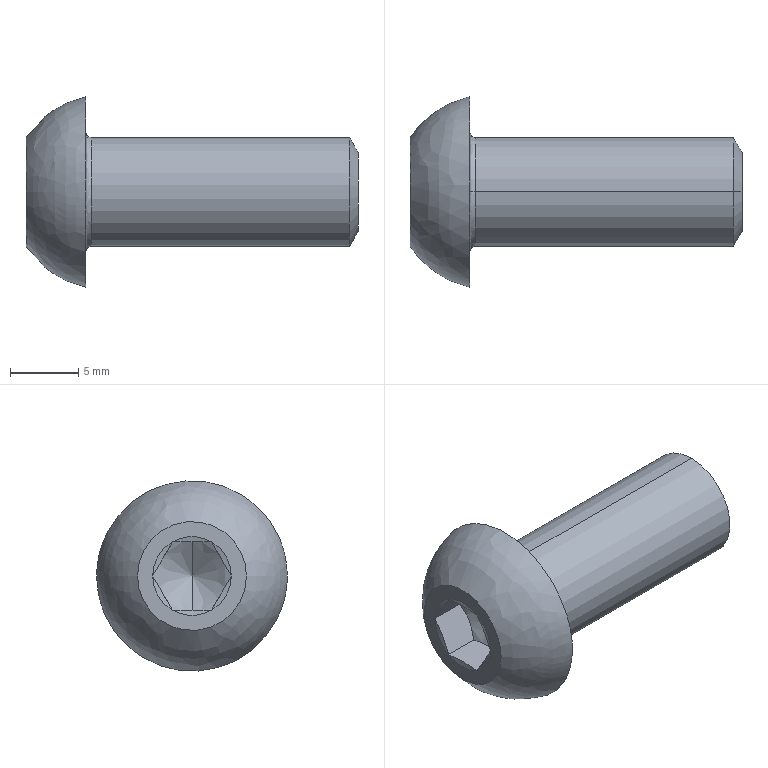Part | SolidWorks | features BaseBody 1 | 1 solid | 24 faces | box 24.4 x 14 x 14 mm | volume 1421 mm3 | cone 10 | plane 9 | spline 3 | cylinder 2 | commonest cylinder face diameters 8 x2
STEP:
#1=CARTESIAN_POINT('',(-19.6,0.,-4.));
#2=VERTEX_POINT('',#1);
#3=CARTESIAN_POINT('',(-19.6,0.,4.));
#4=VERTEX_POINT('',#3);
#5=CARTESIAN_POINT('',(-19.6,0.,0.));
#6=DIRECTION('',(1.,0.,0.));
#7=DIRECTION('',(0.,0.,1.));
#8=AXIS2_PLACEMENT_3D('',#5,#6,#7);
#9=CIRCLE('',#8,4.);
#10=EDGE_CURVE('',#2,#4,#9,.T.);
#11=ORIENTED_EDGE('',*,*,#10,.F.);
#12=CARTESIAN_POINT('',(-20.,0.,-4.4));
#13=VERTEX_POINT('',#12);
#14=CARTESIAN_POINT('',(-19.6,0.,-4.4));
#15=DIRECTION('',(0.,-1.,0.));
#16=DIRECTION('',(0.,0.,-1.));
#17=AXIS2_PLACEMENT_3D('',#14,#15,#16);
#18=CIRCLE('',#17,0.4);
#19=EDGE_CURVE('',#2,#13,#18,.T.);
#20=ORIENTED_EDGE('',*,*,#19,.T.);
#21=CARTESIAN_POINT('',(-20.,0.,4.4));
#22=VERTEX_POINT('',#21);
#23=CARTESIAN_POINT('',(-20.,0.,4.4));
#24=CARTESIAN_POINT('',(-20.,0.2798,4.4));
#25=CARTESIAN_POINT('',(-20.,0.6922,4.361));
#26=CARTESIAN_POINT('',(-20.,1.16,4.249));
#27=CARTESIAN_POINT('',(-20.,1.391,4.176));
#28=CARTESIAN_POINT('',(-20.,1.506,4.135));
#29=CARTESIAN_POINT('',(-20.,1.555,4.116));
#30=CARTESIAN_POINT('',(-20.,1.587,4.104));
#31=CARTESIAN_POINT('',(-20.,1.602,4.098));
#32=CARTESIAN_POINT('',(-20.,1.758,4.036));
#33=CARTESIAN_POINT('',(-20.,1.96,3.944));
#34=CARTESIAN_POINT('',(-20.,2.155,3.837));
#35=CARTESIAN_POINT('',(-20.,2.283,3.762));
#36=CARTESIAN_POINT('',(-20.,2.344,3.724));
#37=CARTESIAN_POINT('',(-20.,2.662,3.516));
#38=CARTESIAN_POINT('',(-20.,2.896,3.326));
#39=CARTESIAN_POINT('',(-20.,3.219,3.004));
#40=CARTESIAN_POINT('',(-20.,3.371,2.835));
#41=CARTESIAN_POINT('',(-20.,3.509,2.656));
#42=CARTESIAN_POINT('',(-20.,3.598,2.533));
#43=CARTESIAN_POINT('',(-20.,3.642,2.47));
#44=CARTESIAN_POINT('',(-20.,3.764,2.283));
#45=CARTESIAN_POINT('',(-20.,3.876,2.091));
#46=CARTESIAN_POINT('',(-20.,3.99,1.858));
#47=CARTESIAN_POINT('',(-20.,4.034,1.757));
#48=CARTESIAN_POINT('',(-20.,4.063,1.688));
#49=CARTESIAN_POINT('',(-20.,4.078,1.652));
#50=CARTESIAN_POINT('',(-20.,4.297,1.099));
#51=CARTESIAN_POINT('',(-20.,4.4,0.5599));
#52=CARTESIAN_POINT('',(-20.,4.4,-0.2799));
#53=CARTESIAN_POINT('',(-20.,4.361,-0.6923));
#54=CARTESIAN_POINT('',(-20.,4.249,-1.16));
#55=CARTESIAN_POINT('',(-20.,4.176,-1.391));
#56=CARTESIAN_POINT('',(-20.,4.135,-1.506));
#57=CARTESIAN_POINT('',(-20.,4.116,-1.555));
#58=CARTESIAN_POINT('',(-20.,4.104,-1.587));
#59=CARTESIAN_POINT('',(-20.,4.098,-1.602));
#60=CARTESIAN_POINT('',(-20.,4.036,-1.758));
#61=CARTESIAN_POINT('',(-20.,3.944,-1.96));
#62=CARTESIAN_POINT('',(-20.,3.837,-2.155));
#63=CARTESIAN_POINT('',(-20.,3.762,-2.283));
#64=CARTESIAN_POINT('',(-20.,3.724,-2.344));
#65=CARTESIAN_POINT('',(-20.,3.516,-2.662));
#66=CARTESIAN_POINT('',(-20.,3.326,-2.896));
#67=CARTESIAN_POINT('',(-20.,3.004,-3.219));
#68=CARTESIAN_POINT('',(-20.,2.835,-3.371));
#69=CARTESIAN_POINT('',(-20.,2.656,-3.509));
#70=CARTESIAN_POINT('',(-20.,2.533,-3.598));
#71=CARTESIAN_POINT('',(-20.,2.47,-3.642));
#72=CARTESIAN_POINT('',(-20.,2.283,-3.764));
#73=CARTESIAN_POINT('',(-20.,2.091,-3.876));
#74=CARTESIAN_POINT('',(-20.,1.858,-3.99));
#75=CARTESIAN_POINT('',(-20.,1.757,-4.034));
#76=CARTESIAN_POINT('',(-20.,1.688,-4.063));
#77=CARTESIAN_POINT('',(-20.,1.652,-4.078));
#78=CARTESIAN_POINT('',(-20.,1.099,-4.297));
#79=CARTESIAN_POINT('',(-20.,0.5593,-4.4));
#80=CARTESIAN_POINT('',(-20.,0.,-4.4));
#81=B_SPLINE_CURVE_WITH_KNOTS('',3,(#23,#24,#25,#26,#27,#28,#29,#30,#31,#32,#33,#34,#35,#36,#37,#38,#39,#40,#41,#42,#43,#44,#45,#46,#47,#48,#49,#50,#51,#52,#53,#54,#55,#56,#57,#58,#59,#60,#61,#62,#63,#64,#65,#66,#67,#68,#69,#70,#71,#72,#73,#74,#75,#76,#77,#78,#79,#80),.UNSPECIFIED.,.F.,.F.,(4,1,1,1,1,2,2,1,2,2,2,1,2,2,1,1,2,2,2,1,1,1,1,2,2,1,2,2,2,1,2,2,1,1,2,2,4),(0.,0.0625,0.09375,0.1094,0.1172,0.1211,0.125,0.1562,0.1719,0.1875,0.25,0.2812,0.2969,0.3125,0.3437,0.3594,0.3672,0.375,0.5,0.5625,0.5937,0.6094,0.6172,0.6211,0.625,0.6562,0.6719,0.6875,0.75,0.7812,0.7969,0.8125,0.8437,0.8594,0.8672,0.875,1.),.UNSPECIFIED.);
#82=EDGE_CURVE('',#22,#13,#81,.T.);
#83=ORIENTED_EDGE('',*,*,#82,.F.);
#84=CARTESIAN_POINT('',(-19.6,0.,4.4));
#85=DIRECTION('',(0.,1.,0.));
#86=DIRECTION('',(0.,0.,1.));
#87=AXIS2_PLACEMENT_3D('',#84,#85,#86);
#88=CIRCLE('',#87,0.4);
#89=EDGE_CURVE('',#4,#22,#88,.T.);
#90=ORIENTED_EDGE('',*,*,#89,.F.);
#91=EDGE_LOOP('',(#11,#20,#83,#90));
#92=FACE_OUTER_BOUND('',#91,.T.);
#93=CARTESIAN_POINT('',(-19.6,0.,4.));
#94=CARTESIAN_POINT('',(-19.6,8.,4.));
#95=CARTESIAN_POINT('',(-19.6,8.,-4.));
#96=CARTESIAN_POINT('',(-19.6,0.,-4.));
#97=CARTESIAN_POINT('',(-19.834,0.,4.));
#98=CARTESIAN_POINT('',(-19.834,8.,4.));
#99=CARTESIAN_POINT('',(-19.834,8.,-4.));
#100=CARTESIAN_POINT('',(-19.834,0.,-4.));
#101=CARTESIAN_POINT('',(-20.,0.,4.166));
#102=CARTESIAN_POINT('',(-20.,8.331,4.166));
#103=CARTESIAN_POINT('',(-20.,8.331,-4.166));
#104=CARTESIAN_POINT('',(-20.,0.,-4.166));
#105=CARTESIAN_POINT('',(-20.,0.,4.4));
#106=CARTESIAN_POINT('',(-20.,8.8,4.4));
#107=CARTESIAN_POINT('',(-20.,8.8,-4.4));
#108=CARTESIAN_POINT('',(-20.,0.,-4.4));
#109=(BOUNDED_SURFACE()B_SPLINE_SURFACE(3,3,((#93,#94,#95,#96),(#97,#98,#99,#100),(#101,#102,#103,#104),(#105,#106,#107,#108)),.UNSPECIFIED.,.F.,.F.,.F.)B_SPLINE_SURFACE_WITH_KNOTS((4,4),(4,4),(0.,1.),(0.,1.),.UNSPECIFIED.)GEOMETRIC_REPRESENTATION_ITEM()RATIONAL_B_SPLINE_SURFACE(((1.,0.3333,0.3333,1.),(0.8047,0.2682,0.2682,0.8047),(0.8047,0.2682,0.2682,0.8047),(1.,0.3333,0.3333,1.)))REPRESENTATION_ITEM('')SURFACE());
#110=ADVANCED_FACE('',(#92),#109,.F.);
#111=CARTESIAN_POINT('',(-0.625,0.,4.));
#112=VERTEX_POINT('',#111);
#113=CARTESIAN_POINT('',(-0.625,0.,-4.));
#114=VERTEX_POINT('',#113);
#115=CARTESIAN_POINT('',(-0.625,0.,0.));
#116=DIRECTION('',(-1.,0.,0.));
#117=DIRECTION('',(0.,0.,1.));
#118=AXIS2_PLACEMENT_3D('',#115,#116,#117);
#119=CIRCLE('',#118,4.);
#120=EDGE_CURVE('',#112,#114,#119,.T.);
#121=ORIENTED_EDGE('',*,*,#120,.T.);
#122=CARTESIAN_POINT('',(-24.4,0.,-4.));
#123=DIRECTION('',(-1.,0.,0.));
#124=VECTOR('',#123,1000.);
#125=LINE('',#122,#124);
#126=EDGE_CURVE('',#114,#2,#125,.T.);
#127=ORIENTED_EDGE('',*,*,#126,.T.);
#128=ORIENTED_EDGE('',*,*,#10,.T.);
#129=CARTESIAN_POINT('',(-24.4,0.,4.));
#130=DIRECTION('',(-1.,0.,0.));
#131=VECTOR('',#130,1000.);
#132=LINE('',#129,#131);
#133=EDGE_CURVE('',#112,#4,#132,.T.);
#134=ORIENTED_EDGE('',*,*,#133,.F.);
#135=EDGE_LOOP('',(#121,#127,#128,#134));
#136=FACE_OUTER_BOUND('',#135,.T.);
#137=CARTESIAN_POINT('',(-24.4,0.,0.));
#138=DIRECTION('',(-1.,0.,0.));
#139=DIRECTION('',(0.,0.,1.));
#140=AXIS2_PLACEMENT_3D('',#137,#138,#139);
#141=CYLINDRICAL_SURFACE('',#140,4.);
#142=ADVANCED_FACE('',(#136),#141,.T.);
#143=CARTESIAN_POINT('',(0.,0.,2.917));
#144=VERTEX_POINT('',#143);
#145=CARTESIAN_POINT('',(0.,0.,-2.917));
#146=VERTEX_POINT('',#145);
#147=CARTESIAN_POINT('',(0.,0.,0.));
#148=DIRECTION('',(-1.,0.,0.));
#149=DIRECTION('',(0.,0.,1.));
#150=AXIS2_PLACEMENT_3D('',#147,#148,#149);
#151=CIRCLE('',#150,2.917);
#152=EDGE_CURVE('',#144,#146,#151,.T.);
#153=ORIENTED_EDGE('',*,*,#152,.T.);
#154=CARTESIAN_POINT('',(-0.625,0.,-4.));
#155=DIRECTION('',(-0.5,0.,-0.866));
#156=VECTOR('',#155,1000.);
#157=LINE('',#154,#156);
#158=EDGE_CURVE('',#146,#114,#157,.T.);
#159=ORIENTED_EDGE('',*,*,#158,.T.);
#160=ORIENTED_EDGE('',*,*,#120,.F.);
#161=CARTESIAN_POINT('',(-0.625,0.,4.));
#162=DIRECTION('',(-0.5,0.,0.866));
#163=VECTOR('',#162,1000.);
#164=LINE('',#161,#163);
#165=EDGE_CURVE('',#144,#112,#164,.T.);
#166=ORIENTED_EDGE('',*,*,#165,.F.);
#167=EDGE_LOOP('',(#153,#159,#160,#166));
#168=FACE_OUTER_BOUND('',#167,.T.);
#169=CARTESIAN_POINT('',(-0.625,0.,0.));
#170=DIRECTION('',(-1.,0.,0.));
#171=DIRECTION('',(0.,0.,1.));
#172=AXIS2_PLACEMENT_3D('',#169,#170,#171);
#173=CONICAL_SURFACE('',#172,4.,1.047);
#174=ADVANCED_FACE('',(#168),#173,.T.);
#175=CARTESIAN_POINT('',(-20.,0.,0.));
#176=VERTEX_POINT('',#175);
#177=CARTESIAN_POINT('',(-21.559,0.,2.5));
#178=VERTEX_POINT('',#177);
#179=CARTESIAN_POINT('',(-21.811,0.,2.904));
#180=DIRECTION('',(-0.5291,0.,0.8486));
#181=VECTOR('',#180,1000.);
#182=LINE('',#179,#181);
#183=EDGE_CURVE('',#176,#178,#182,.T.);
#184=ORIENTED_EDGE('',*,*,#183,.F.);
#185=CARTESIAN_POINT('',(-21.559,0.,-2.5));
#186=VERTEX_POINT('',#185);
#187=CARTESIAN_POINT('',(-21.811,0.,-2.904));
#188=DIRECTION('',(-0.5291,0.,-0.8486));
#189=VECTOR('',#188,1000.);
#190=LINE('',#187,#189);
#191=EDGE_CURVE('',#176,#186,#190,.T.);
#192=ORIENTED_EDGE('',*,*,#191,.T.);
#193=CARTESIAN_POINT('',(-21.8,-1.443,-2.5));
#194=VERTEX_POINT('',#193);
#195=CARTESIAN_POINT('',(-21.559,0.,-2.5));
#196=CARTESIAN_POINT('',(-21.559,-0.4946,-2.5));
#197=CARTESIAN_POINT('',(-21.653,-0.9733,-2.5));
#198=CARTESIAN_POINT('',(-21.8,-1.443,-2.5));
#199=B_SPLINE_CURVE_WITH_KNOTS('',3,(#195,#196,#197,#198),.UNSPECIFIED.,.F.,.F.,(4,4),(0.,0.001463),.UNSPECIFIED.);
#200=EDGE_CURVE('',#186,#194,#199,.T.);
#201=ORIENTED_EDGE('',*,*,#200,.T.);
#202=CARTESIAN_POINT('',(-21.8,-2.887,0.));
#203=VERTEX_POINT('',#202);
#204=CARTESIAN_POINT('',(-21.8,-1.443,-2.5));
#205=CARTESIAN_POINT('',(-21.654,-1.678,-2.093));
#206=CARTESIAN_POINT('',(-21.559,-1.917,-1.679));
#207=CARTESIAN_POINT('',(-21.559,-2.286,-1.04));
#208=CARTESIAN_POINT('',(-21.582,-2.409,-0.8268));
#209=CARTESIAN_POINT('',(-21.666,-2.65,-0.4095));
#210=CARTESIAN_POINT('',(-21.727,-2.769,-0.2038));
#211=CARTESIAN_POINT('',(-21.8,-2.887,0.));
#212=B_SPLINE_CURVE_WITH_KNOTS('',3,(#204,#205,#206,#207,#208,#209,#210,#211),.UNSPECIFIED.,.F.,.F.,(4,2,2,4),(0.,0.00146,0.002189,0.002919),.UNSPECIFIED.);
#213=EDGE_CURVE('',#194,#203,#212,.T.);
#214=ORIENTED_EDGE('',*,*,#213,.T.);
#215=CARTESIAN_POINT('',(-21.8,-1.443,2.5));
#216=VERTEX_POINT('',#215);
#217=CARTESIAN_POINT('',(-21.8,-2.887,0.));
#218=CARTESIAN_POINT('',(-21.654,-2.652,0.4068));
#219=CARTESIAN_POINT('',(-21.559,-2.413,0.8206));
#220=CARTESIAN_POINT('',(-21.559,-2.044,1.46));
#221=CARTESIAN_POINT('',(-21.582,-1.921,1.673));
#222=CARTESIAN_POINT('',(-21.666,-1.68,2.09));
#223=CARTESIAN_POINT('',(-21.727,-1.561,2.296));
#224=CARTESIAN_POINT('',(-21.8,-1.443,2.5));
#225=B_SPLINE_CURVE_WITH_KNOTS('',3,(#217,#218,#219,#220,#221,#222,#223,#224),.UNSPECIFIED.,.F.,.F.,(4,2,2,4),(0.,0.00146,0.002189,0.002919),.UNSPECIFIED.);
#226=EDGE_CURVE('',#203,#216,#225,.T.);
#227=ORIENTED_EDGE('',*,*,#226,.T.);
#228=CARTESIAN_POINT('',(-21.559,0.,2.5));
#229=CARTESIAN_POINT('',(-21.559,-0.4946,2.5));
#230=CARTESIAN_POINT('',(-21.653,-0.9733,2.5));
#231=CARTESIAN_POINT('',(-21.8,-1.443,2.5));
#232=B_SPLINE_CURVE_WITH_KNOTS('',3,(#228,#229,#230,#231),.UNSPECIFIED.,.F.,.F.,(4,4),(0.,0.001463),.UNSPECIFIED.);
#233=EDGE_CURVE('',#178,#216,#232,.T.);
#234=ORIENTED_EDGE('',*,*,#233,.F.);
#235=EDGE_LOOP('',(#184,#192,#201,#214,#227,#234));
#236=FACE_OUTER_BOUND('',#235,.T.);
#237=CARTESIAN_POINT('',(-21.811,0.,0.));
#238=DIRECTION('',(-1.,0.,0.));
#239=DIRECTION('',(0.,0.,1.));
#240=AXIS2_PLACEMENT_3D('',#237,#238,#239);
#241=CONICAL_SURFACE('',#240,2.904,1.013);
#242=ADVANCED_FACE('',(#236),#241,.F.);
#243=ORIENTED_EDGE('',*,*,#126,.F.);
#244=CARTESIAN_POINT('',(-0.625,0.,0.));
#245=DIRECTION('',(-1.,0.,0.));
#246=DIRECTION('',(0.,0.,1.));
#247=AXIS2_PLACEMENT_3D('',#244,#245,#246);
#248=CIRCLE('',#247,4.);
#249=EDGE_CURVE('',#114,#112,#248,.T.);
#250=ORIENTED_EDGE('',*,*,#249,.T.);
#251=ORIENTED_EDGE('',*,*,#133,.T.);
#252=CARTESIAN_POINT('',(-19.6,0.,0.));
#253=DIRECTION('',(1.,0.,0.));
#254=DIRECTION('',(0.,0.,1.));
#255=AXIS2_PLACEMENT_3D('',#252,#253,#254);
#256=CIRCLE('',#255,4.);
#257=EDGE_CURVE('',#4,#2,#256,.T.);
#258=ORIENTED_EDGE('',*,*,#257,.T.);
#259=EDGE_LOOP('',(#243,#250,#251,#258));
#260=FACE_OUTER_BOUND('',#259,.T.);
#261=CARTESIAN_POINT('',(-24.4,0.,0.));
#262=DIRECTION('',(-1.,0.,0.));
#263=DIRECTION('',(0.,0.,1.));
#264=AXIS2_PLACEMENT_3D('',#261,#262,#263);
#265=CYLINDRICAL_SURFACE('',#264,4.);
#266=ADVANCED_FACE('',(#260),#265,.T.);
#267=ORIENTED_EDGE('',*,*,#19,.F.);
#268=ORIENTED_EDGE('',*,*,#257,.F.);
#269=ORIENTED_EDGE('',*,*,#89,.T.);
#270=CARTESIAN_POINT('',(-20.,0.,-4.4));
#271=CARTESIAN_POINT('',(-20.,-0.2798,-4.4));
#272=CARTESIAN_POINT('',(-20.,-0.6922,-4.361));
#273=CARTESIAN_POINT('',(-20.,-1.16,-4.249));
#274=CARTESIAN_POINT('',(-20.,-1.391,-4.176));
#275=CARTESIAN_POINT('',(-20.,-1.506,-4.135));
#276=CARTESIAN_POINT('',(-20.,-1.555,-4.116));
#277=CARTESIAN_POINT('',(-20.,-1.587,-4.104));
#278=CARTESIAN_POINT('',(-20.,-1.602,-4.098));
#279=CARTESIAN_POINT('',(-20.,-1.758,-4.036));
#280=CARTESIAN_POINT('',(-20.,-1.96,-3.944));
#281=CARTESIAN_POINT('',(-20.,-2.155,-3.837));
#282=CARTESIAN_POINT('',(-20.,-2.283,-3.762));
#283=CARTESIAN_POINT('',(-20.,-2.344,-3.724));
#284=CARTESIAN_POINT('',(-20.,-2.662,-3.516));
#285=CARTESIAN_POINT('',(-20.,-2.896,-3.326));
#286=CARTESIAN_POINT('',(-20.,-3.219,-3.004));
#287=CARTESIAN_POINT('',(-20.,-3.371,-2.835));
#288=CARTESIAN_POINT('',(-20.,-3.509,-2.656));
#289=CARTESIAN_POINT('',(-20.,-3.598,-2.533));
#290=CARTESIAN_POINT('',(-20.,-3.642,-2.47));
#291=CARTESIAN_POINT('',(-20.,-3.764,-2.283));
#292=CARTESIAN_POINT('',(-20.,-3.876,-2.091));
#293=CARTESIAN_POINT('',(-20.,-3.99,-1.858));
#294=CARTESIAN_POINT('',(-20.,-4.034,-1.757));
#295=CARTESIAN_POINT('',(-20.,-4.063,-1.688));
#296=CARTESIAN_POINT('',(-20.,-4.078,-1.652));
#297=CARTESIAN_POINT('',(-20.,-4.297,-1.099));
#298=CARTESIAN_POINT('',(-20.,-4.4,-0.5599));
#299=CARTESIAN_POINT('',(-20.,-4.4,0.2799));
#300=CARTESIAN_POINT('',(-20.,-4.361,0.6923));
#301=CARTESIAN_POINT('',(-20.,-4.249,1.16));
#302=CARTESIAN_POINT('',(-20.,-4.176,1.391));
#303=CARTESIAN_POINT('',(-20.,-4.135,1.506));
#304=CARTESIAN_POINT('',(-20.,-4.116,1.555));
#305=CARTESIAN_POINT('',(-20.,-4.104,1.587));
#306=CARTESIAN_POINT('',(-20.,-4.098,1.602));
#307=CARTESIAN_POINT('',(-20.,-4.036,1.758));
#308=CARTESIAN_POINT('',(-20.,-3.944,1.96));
#309=CARTESIAN_POINT('',(-20.,-3.837,2.155));
#310=CARTESIAN_POINT('',(-20.,-3.762,2.283));
#311=CARTESIAN_POINT('',(-20.,-3.724,2.344));
#312=CARTESIAN_POINT('',(-20.,-3.516,2.662));
#313=CARTESIAN_POINT('',(-20.,-3.326,2.896));
#314=CARTESIAN_POINT('',(-20.,-3.004,3.219));
#315=CARTESIAN_POINT('',(-20.,-2.835,3.371));
#316=CARTESIAN_POINT('',(-20.,-2.656,3.509));
#317=CARTESIAN_POINT('',(-20.,-2.533,3.598));
#318=CARTESIAN_POINT('',(-20.,-2.47,3.642));
#319=CARTESIAN_POINT('',(-20.,-2.283,3.764));
#320=CARTESIAN_POINT('',(-20.,-2.091,3.876));
#321=CARTESIAN_POINT('',(-20.,-1.858,3.99));
#322=CARTESIAN_POINT('',(-20.,-1.757,4.034));
#323=CARTESIAN_POINT('',(-20.,-1.688,4.063));
#324=CARTESIAN_POINT('',(-20.,-1.652,4.078));
#325=CARTESIAN_POINT('',(-20.,-1.099,4.297));
#326=CARTESIAN_POINT('',(-20.,-0.5593,4.4));
#327=CARTESIAN_POINT('',(-20.,0.,4.4));
#328=B_SPLINE_CURVE_WITH_KNOTS('',3,(#270,#271,#272,#273,#274,#275,#276,#277,#278,#279,#280,#281,#282,#283,#284,#285,#286,#287,#288,#289,#290,#291,#292,#293,#294,#295,#296,#297,#298,#299,#300,#301,#302,#303,#304,#305,#306,#307,#308,#309,#310,#311,#312,#313,#314,#315,#316,#317,#318,#319,#320,#321,#322,#323,#324,#325,#326,#327),.UNSPECIFIED.,.F.,.F.,(4,1,1,1,1,2,2,1,2,2,2,1,2,2,1,1,2,2,2,1,1,1,1,2,2,1,2,2,2,1,2,2,1,1,2,2,4),(0.,0.0625,0.09375,0.1094,0.1172,0.1211,0.125,0.1562,0.1719,0.1875,0.25,0.2812,0.2969,0.3125,0.3437,0.3594,0.3672,0.375,0.5,0.5625,0.5937,0.6094,0.6172,0.6211,0.625,0.6562,0.6719,0.6875,0.75,0.7812,0.7969,0.8125,0.8437,0.8594,0.8672,0.875,1.),.UNSPECIFIED.);
#329=EDGE_CURVE('',#13,#22,#328,.T.);
#330=ORIENTED_EDGE('',*,*,#329,.F.);
#331=EDGE_LOOP('',(#267,#268,#269,#330));
#332=FACE_OUTER_BOUND('',#331,.T.);
#333=CARTESIAN_POINT('',(-19.6,0.,-4.));
#334=CARTESIAN_POINT('',(-19.6,-8.,-4.));
#335=CARTESIAN_POINT('',(-19.6,-8.,4.));
#336=CARTESIAN_POINT('',(-19.6,0.,4.));
#337=CARTESIAN_POINT('',(-19.834,0.,-4.));
#338=CARTESIAN_POINT('',(-19.834,-8.,-4.));
#339=CARTESIAN_POINT('',(-19.834,-8.,4.));
#340=CARTESIAN_POINT('',(-19.834,0.,4.));
#341=CARTESIAN_POINT('',(-20.,0.,-4.166));
#342=CARTESIAN_POINT('',(-20.,-8.331,-4.166));
#343=CARTESIAN_POINT('',(-20.,-8.331,4.166));
#344=CARTESIAN_POINT('',(-20.,0.,4.166));
#345=CARTESIAN_POINT('',(-20.,0.,-4.4));
#346=CARTESIAN_POINT('',(-20.,-8.8,-4.4));
#347=CARTESIAN_POINT('',(-20.,-8.8,4.4));
#348=CARTESIAN_POINT('',(-20.,0.,4.4));
#349=(BOUNDED_SURFACE()B_SPLINE_SURFACE(3,3,((#333,#334,#335,#336),(#337,#338,#339,#340),(#341,#342,#343,#344),(#345,#346,#347,#348)),.UNSPECIFIED.,.F.,.F.,.F.)B_SPLINE_SURFACE_WITH_KNOTS((4,4),(4,4),(0.,1.),(0.,1.),.UNSPECIFIED.)GEOMETRIC_REPRESENTATION_ITEM()RATIONAL_B_SPLINE_SURFACE(((1.,0.3333,0.3333,1.),(0.8047,0.2682,0.2682,0.8047),(0.8047,0.2682,0.2682,0.8047),(1.,0.3333,0.3333,1.)))REPRESENTATION_ITEM('')SURFACE());
#350=ADVANCED_FACE('',(#332),#349,.F.);
#351=ORIENTED_EDGE('',*,*,#158,.F.);
#352=CARTESIAN_POINT('',(0.,0.,0.));
#353=DIRECTION('',(-1.,0.,0.));
#354=DIRECTION('',(0.,0.,1.));
#355=AXIS2_PLACEMENT_3D('',#352,#353,#354);
#356=CIRCLE('',#355,2.917);
#357=EDGE_CURVE('',#146,#144,#356,.T.);
#358=ORIENTED_EDGE('',*,*,#357,.T.);
#359=ORIENTED_EDGE('',*,*,#165,.T.);
#360=ORIENTED_EDGE('',*,*,#249,.F.);
#361=EDGE_LOOP('',(#351,#358,#359,#360));
#362=FACE_OUTER_BOUND('',#361,.T.);
#363=CARTESIAN_POINT('',(-0.625,0.,0.));
#364=DIRECTION('',(-1.,0.,0.));
#365=DIRECTION('',(0.,0.,1.));
#366=AXIS2_PLACEMENT_3D('',#363,#364,#365);
#367=CONICAL_SURFACE('',#366,4.,1.047);
#368=ADVANCED_FACE('',(#362),#367,.T.);
#369=ORIENTED_EDGE('',*,*,#329,.T.);
#370=ORIENTED_EDGE('',*,*,#82,.T.);
#371=EDGE_LOOP('',(#369,#370));
#372=FACE_BOUND('',#371,.T.);
#373=CARTESIAN_POINT('',(-20.,7.,0.));
#374=VERTEX_POINT('',#373);
#375=CARTESIAN_POINT('',(-20.,-7.,0.));
#376=VERTEX_POINT('',#375);
#377=CARTESIAN_POINT('',(-20.,7.,0.));
#378=CARTESIAN_POINT('',(-20.,7.,-0.4622));
#379=CARTESIAN_POINT('',(-20.,6.955,-0.9197));
#380=CARTESIAN_POINT('',(-20.,6.774,-1.825));
#381=CARTESIAN_POINT('',(-20.,6.64,-2.263));
#382=CARTESIAN_POINT('',(-20.,6.378,-2.895));
#383=CARTESIAN_POINT('',(-20.,6.28,-3.101));
#384=CARTESIAN_POINT('',(-20.,6.063,-3.506));
#385=CARTESIAN_POINT('',(-20.,5.944,-3.704));
#386=CARTESIAN_POINT('',(-20.,5.561,-4.277));
#387=CARTESIAN_POINT('',(-20.,5.271,-4.629));
#388=CARTESIAN_POINT('',(-20.,4.625,-5.274));
#389=CARTESIAN_POINT('',(-20.,4.264,-5.57));
#390=CARTESIAN_POINT('',(-20.,3.505,-6.077));
#391=CARTESIAN_POINT('',(-20.,3.103,-6.292));
#392=CARTESIAN_POINT('',(-20.,2.466,-6.555));
#393=CARTESIAN_POINT('',(-20.,2.248,-6.633));
#394=CARTESIAN_POINT('',(-20.,1.809,-6.766));
#395=CARTESIAN_POINT('',(-20.,1.587,-6.821));
#396=CARTESIAN_POINT('',(-20.,0.917,-6.955));
#397=CARTESIAN_POINT('',(-20.,0.4599,-7.));
#398=CARTESIAN_POINT('',(-20.,-0.4622,-7.));
#399=CARTESIAN_POINT('',(-20.,-0.9163,-6.955));
#400=CARTESIAN_POINT('',(-20.,-1.587,-6.821));
#401=CARTESIAN_POINT('',(-20.,-1.809,-6.766));
#402=CARTESIAN_POINT('',(-20.,-2.25,-6.633));
#403=CARTESIAN_POINT('',(-20.,-2.468,-6.555));
#404=CARTESIAN_POINT('',(-20.,-3.102,-6.292));
#405=CARTESIAN_POINT('',(-20.,-3.504,-6.077));
#406=CARTESIAN_POINT('',(-20.,-4.075,-5.696));
#407=CARTESIAN_POINT('',(-20.,-4.261,-5.558));
#408=CARTESIAN_POINT('',(-20.,-4.617,-5.266));
#409=CARTESIAN_POINT('',(-20.,-4.787,-5.113));
#410=CARTESIAN_POINT('',(-20.,-5.271,-4.629));
#411=CARTESIAN_POINT('',(-20.,-5.561,-4.277));
#412=CARTESIAN_POINT('',(-20.,-6.073,-3.511));
#413=CARTESIAN_POINT('',(-20.,-6.29,-3.105));
#414=CARTESIAN_POINT('',(-20.,-6.552,-2.474));
#415=CARTESIAN_POINT('',(-20.,-6.629,-2.259));
#416=CARTESIAN_POINT('',(-20.,-6.763,-1.821));
#417=CARTESIAN_POINT('',(-20.,-6.819,-1.596));
#418=CARTESIAN_POINT('',(-20.,-6.955,-0.919));
#419=CARTESIAN_POINT('',(-20.,-7.,-0.4622));
#420=CARTESIAN_POINT('',(-20.,-7.,0.));
#421=B_SPLINE_CURVE_WITH_KNOTS('',3,(#377,#378,#379,#380,#381,#382,#383,#384,#385,#386,#387,#388,#389,#390,#391,#392,#393,#394,#395,#396,#397,#398,#399,#400,#401,#402,#403,#404,#405,#406,#407,#408,#409,#410,#411,#412,#413,#414,#415,#416,#417,#418,#419,#420),.UNSPECIFIED.,.F.,.F.,(4,2,2,2,2,2,2,2,2,2,2,2,2,2,2,2,2,2,2,2,2,4),(0.,0.001379,0.002758,0.003448,0.004138,0.005517,0.006896,0.008275,0.008965,0.009654,0.01103,0.01241,0.0131,0.01379,0.01517,0.01586,0.01655,0.01793,0.01931,0.02,0.02069,0.02207),.UNSPECIFIED.);
#422=EDGE_CURVE('',#374,#376,#421,.T.);
#423=ORIENTED_EDGE('',*,*,#422,.F.);
#424=CARTESIAN_POINT('',(-20.,-7.,0.));
#425=CARTESIAN_POINT('',(-20.,-7.,0.4622));
#426=CARTESIAN_POINT('',(-20.,-6.955,0.9197));
#427=CARTESIAN_POINT('',(-20.,-6.774,1.825));
#428=CARTESIAN_POINT('',(-20.,-6.64,2.263));
#429=CARTESIAN_POINT('',(-20.,-6.378,2.895));
#430=CARTESIAN_POINT('',(-20.,-6.28,3.101));
#431=CARTESIAN_POINT('',(-20.,-6.063,3.506));
#432=CARTESIAN_POINT('',(-20.,-5.944,3.704));
#433=CARTESIAN_POINT('',(-20.,-5.561,4.277));
#434=CARTESIAN_POINT('',(-20.,-5.271,4.629));
#435=CARTESIAN_POINT('',(-20.,-4.625,5.274));
#436=CARTESIAN_POINT('',(-20.,-4.264,5.57));
#437=CARTESIAN_POINT('',(-20.,-3.505,6.077));
#438=CARTESIAN_POINT('',(-20.,-3.103,6.292));
#439=CARTESIAN_POINT('',(-20.,-2.466,6.555));
#440=CARTESIAN_POINT('',(-20.,-2.248,6.633));
#441=CARTESIAN_POINT('',(-20.,-1.809,6.766));
#442=CARTESIAN_POINT('',(-20.,-1.587,6.821));
#443=CARTESIAN_POINT('',(-20.,-0.917,6.955));
#444=CARTESIAN_POINT('',(-20.,-0.4599,7.));
#445=CARTESIAN_POINT('',(-20.,0.4622,7.));
#446=CARTESIAN_POINT('',(-20.,0.9163,6.955));
#447=CARTESIAN_POINT('',(-20.,1.587,6.821));
#448=CARTESIAN_POINT('',(-20.,1.809,6.766));
#449=CARTESIAN_POINT('',(-20.,2.25,6.633));
#450=CARTESIAN_POINT('',(-20.,2.468,6.555));
#451=CARTESIAN_POINT('',(-20.,3.102,6.292));
#452=CARTESIAN_POINT('',(-20.,3.504,6.077));
#453=CARTESIAN_POINT('',(-20.,4.075,5.696));
#454=CARTESIAN_POINT('',(-20.,4.261,5.558));
#455=CARTESIAN_POINT('',(-20.,4.617,5.266));
#456=CARTESIAN_POINT('',(-20.,4.787,5.113));
#457=CARTESIAN_POINT('',(-20.,5.271,4.629));
#458=CARTESIAN_POINT('',(-20.,5.561,4.277));
#459=CARTESIAN_POINT('',(-20.,6.073,3.511));
#460=CARTESIAN_POINT('',(-20.,6.29,3.105));
#461=CARTESIAN_POINT('',(-20.,6.552,2.474));
#462=CARTESIAN_POINT('',(-20.,6.629,2.259));
#463=CARTESIAN_POINT('',(-20.,6.763,1.821));
#464=CARTESIAN_POINT('',(-20.,6.819,1.596));
#465=CARTESIAN_POINT('',(-20.,6.955,0.919));
#466=CARTESIAN_POINT('',(-20.,7.,0.4622));
#467=CARTESIAN_POINT('',(-20.,7.,0.));
#468=B_SPLINE_CURVE_WITH_KNOTS('',3,(#424,#425,#426,#427,#428,#429,#430,#431,#432,#433,#434,#435,#436,#437,#438,#439,#440,#441,#442,#443,#444,#445,#446,#447,#448,#449,#450,#451,#452,#453,#454,#455,#456,#457,#458,#459,#460,#461,#462,#463,#464,#465,#466,#467),.UNSPECIFIED.,.F.,.F.,(4,2,2,2,2,2,2,2,2,2,2,2,2,2,2,2,2,2,2,2,2,4),(0.02207,0.02345,0.02483,0.02552,0.0262,0.02758,0.02896,0.03034,0.03103,0.03172,0.0331,0.03448,0.03517,0.03586,0.03724,0.03793,0.03862,0.04,0.04138,0.04207,0.04276,0.04413),.UNSPECIFIED.);
#469=EDGE_CURVE('',#376,#374,#468,.T.);
#470=ORIENTED_EDGE('',*,*,#469,.F.);
#471=EDGE_LOOP('',(#423,#470));
#472=FACE_OUTER_BOUND('',#471,.T.);
#473=CARTESIAN_POINT('',(-20.,4.4,0.));
#474=DIRECTION('',(-1.,0.,0.));
#475=DIRECTION('',(0.,0.,1.));
#476=AXIS2_PLACEMENT_3D('',#473,#474,#475);
#477=PLANE('',#476);
#478=ADVANCED_FACE('',(#372,#472),#477,.F.);
#479=ORIENTED_EDGE('',*,*,#152,.F.);
#480=ORIENTED_EDGE('',*,*,#357,.F.);
#481=EDGE_LOOP('',(#479,#480));
#482=FACE_OUTER_BOUND('',#481,.T.);
#483=CARTESIAN_POINT('',(0.,4.,0.));
#484=DIRECTION('',(-1.,0.,0.));
#485=DIRECTION('',(0.,0.,1.));
#486=AXIS2_PLACEMENT_3D('',#483,#484,#485);
#487=PLANE('',#486);
#488=ADVANCED_FACE('',(#482),#487,.F.);
#489=CARTESIAN_POINT('',(-24.4,-4.,0.));
#490=VERTEX_POINT('',#489);
#491=CARTESIAN_POINT('',(-24.4,4.,0.));
#492=VERTEX_POINT('',#491);
#493=CARTESIAN_POINT('',(-24.4,-4.,0.));
#494=CARTESIAN_POINT('',(-24.4,-4.,-0.2642));
#495=CARTESIAN_POINT('',(-24.4,-3.974,-0.5241));
#496=CARTESIAN_POINT('',(-24.4,-3.872,-1.035));
#497=CARTESIAN_POINT('',(-24.4,-3.796,-1.289));
#498=CARTESIAN_POINT('',(-24.4,-3.595,-1.774));
#499=CARTESIAN_POINT('',(-24.4,-3.472,-2.003));
#500=CARTESIAN_POINT('',(-24.4,-3.182,-2.438));
#501=CARTESIAN_POINT('',(-24.4,-3.013,-2.644));
#502=CARTESIAN_POINT('',(-24.4,-2.644,-3.013));
#503=CARTESIAN_POINT('',(-24.4,-2.443,-3.179));
#504=CARTESIAN_POINT('',(-24.4,-2.005,-3.471));
#505=CARTESIAN_POINT('',(-24.4,-1.773,-3.595));
#506=CARTESIAN_POINT('',(-24.4,-1.291,-3.795));
#507=CARTESIAN_POINT('',(-24.4,-1.039,-3.872));
#508=CARTESIAN_POINT('',(-24.4,-0.523,-3.974));
#509=CARTESIAN_POINT('',(-24.4,-0.2635,-4.));
#510=CARTESIAN_POINT('',(-24.4,0.2581,-4.));
#511=CARTESIAN_POINT('',(-24.4,0.5231,-3.974));
#512=CARTESIAN_POINT('',(-24.4,1.036,-3.872));
#513=CARTESIAN_POINT('',(-24.4,1.285,-3.797));
#514=CARTESIAN_POINT('',(-24.4,1.77,-3.597));
#515=CARTESIAN_POINT('',(-24.4,2.004,-3.472));
#516=CARTESIAN_POINT('',(-24.4,2.437,-3.182));
#517=CARTESIAN_POINT('',(-24.4,2.64,-3.017));
#518=CARTESIAN_POINT('',(-24.4,3.013,-2.644));
#519=CARTESIAN_POINT('',(-24.4,3.179,-2.442));
#520=CARTESIAN_POINT('',(-24.4,3.469,-2.009));
#521=CARTESIAN_POINT('',(-24.4,3.594,-1.775));
#522=CARTESIAN_POINT('',(-24.4,3.795,-1.29));
#523=CARTESIAN_POINT('',(-24.4,3.871,-1.041));
#524=CARTESIAN_POINT('',(-24.4,3.974,-0.5286));
#525=CARTESIAN_POINT('',(-24.4,4.,-0.2642));
#526=CARTESIAN_POINT('',(-24.4,4.,0.));
#527=B_SPLINE_CURVE_WITH_KNOTS('',3,(#493,#494,#495,#496,#497,#498,#499,#500,#501,#502,#503,#504,#505,#506,#507,#508,#509,#510,#511,#512,#513,#514,#515,#516,#517,#518,#519,#520,#521,#522,#523,#524,#525,#526),.UNSPECIFIED.,.F.,.F.,(4,2,2,2,2,2,2,2,2,2,2,2,2,2,2,2,4),(0.,0.0007815,0.001563,0.002344,0.003126,0.003907,0.004689,0.00547,0.006252,0.007033,0.007815,0.008596,0.009377,0.01016,0.01094,0.01172,0.0125),.UNSPECIFIED.);
#528=EDGE_CURVE('',#490,#492,#527,.T.);
#529=ORIENTED_EDGE('',*,*,#528,.T.);
#530=CARTESIAN_POINT('',(-24.4,4.,0.));
#531=CARTESIAN_POINT('',(-24.4,4.,0.2642));
#532=CARTESIAN_POINT('',(-24.4,3.974,0.5241));
#533=CARTESIAN_POINT('',(-24.4,3.872,1.035));
#534=CARTESIAN_POINT('',(-24.4,3.796,1.289));
#535=CARTESIAN_POINT('',(-24.4,3.595,1.774));
#536=CARTESIAN_POINT('',(-24.4,3.472,2.003));
#537=CARTESIAN_POINT('',(-24.4,3.182,2.438));
#538=CARTESIAN_POINT('',(-24.4,3.013,2.644));
#539=CARTESIAN_POINT('',(-24.4,2.644,3.013));
#540=CARTESIAN_POINT('',(-24.4,2.443,3.179));
#541=CARTESIAN_POINT('',(-24.4,2.005,3.471));
#542=CARTESIAN_POINT('',(-24.4,1.773,3.595));
#543=CARTESIAN_POINT('',(-24.4,1.291,3.795));
#544=CARTESIAN_POINT('',(-24.4,1.039,3.872));
#545=CARTESIAN_POINT('',(-24.4,0.523,3.974));
#546=CARTESIAN_POINT('',(-24.4,0.2635,4.));
#547=CARTESIAN_POINT('',(-24.4,-0.2581,4.));
#548=CARTESIAN_POINT('',(-24.4,-0.5231,3.974));
#549=CARTESIAN_POINT('',(-24.4,-1.036,3.872));
#550=CARTESIAN_POINT('',(-24.4,-1.285,3.797));
#551=CARTESIAN_POINT('',(-24.4,-1.77,3.597));
#552=CARTESIAN_POINT('',(-24.4,-2.004,3.472));
#553=CARTESIAN_POINT('',(-24.4,-2.437,3.182));
#554=CARTESIAN_POINT('',(-24.4,-2.64,3.017));
#555=CARTESIAN_POINT('',(-24.4,-3.013,2.644));
#556=CARTESIAN_POINT('',(-24.4,-3.179,2.442));
#557=CARTESIAN_POINT('',(-24.4,-3.469,2.009));
#558=CARTESIAN_POINT('',(-24.4,-3.594,1.775));
#559=CARTESIAN_POINT('',(-24.4,-3.795,1.29));
#560=CARTESIAN_POINT('',(-24.4,-3.871,1.041));
#561=CARTESIAN_POINT('',(-24.4,-3.974,0.5286));
#562=CARTESIAN_POINT('',(-24.4,-4.,0.2642));
#563=CARTESIAN_POINT('',(-24.4,-4.,0.));
#564=B_SPLINE_CURVE_WITH_KNOTS('',3,(#530,#531,#532,#533,#534,#535,#536,#537,#538,#539,#540,#541,#542,#543,#544,#545,#546,#547,#548,#549,#550,#551,#552,#553,#554,#555,#556,#557,#558,#559,#560,#561,#562,#563),.UNSPECIFIED.,.F.,.F.,(4,2,2,2,2,2,2,2,2,2,2,2,2,2,2,2,4),(0.0125,0.01328,0.01407,0.01485,0.01563,0.01641,0.01719,0.01797,0.01875,0.01954,0.02032,0.0211,0.02188,0.02266,0.02344,0.02423,0.02501),.UNSPECIFIED.);
#565=EDGE_CURVE('',#492,#490,#564,.T.);
#566=ORIENTED_EDGE('',*,*,#565,.T.);
#567=EDGE_LOOP('',(#529,#566));
#568=FACE_BOUND('',#567,.T.);
#569=ORIENTED_EDGE('',*,*,#422,.T.);
#570=ORIENTED_EDGE('',*,*,#469,.T.);
#571=EDGE_LOOP('',(#569,#570));
#572=FACE_OUTER_BOUND('',#571,.T.);
#573=CARTESIAN_POINT('',(-18.737,7.024,-1.407));
#574=CARTESIAN_POINT('',(-20.707,7.024,-1.005));
#575=CARTESIAN_POINT('',(-20.707,7.024,1.005));
#576=CARTESIAN_POINT('',(-18.737,7.024,1.407));
#577=CARTESIAN_POINT('',(-20.702,5.015,-11.035));
#578=CARTESIAN_POINT('',(-36.149,5.015,-7.883));
#579=CARTESIAN_POINT('',(-36.149,5.015,7.883));
#580=CARTESIAN_POINT('',(-20.702,5.015,11.035));
#581=CARTESIAN_POINT('',(-20.702,-5.015,-11.035));
#582=CARTESIAN_POINT('',(-36.149,-5.015,-7.883));
#583=CARTESIAN_POINT('',(-36.149,-5.015,7.883));
#584=CARTESIAN_POINT('',(-20.702,-5.015,11.035));
#585=CARTESIAN_POINT('',(-18.737,-7.024,-1.407));
#586=CARTESIAN_POINT('',(-20.707,-7.024,-1.005));
#587=CARTESIAN_POINT('',(-20.707,-7.024,1.005));
#588=CARTESIAN_POINT('',(-18.737,-7.024,1.407));
#589=(BOUNDED_SURFACE()B_SPLINE_SURFACE(3,3,((#573,#574,#575,#576),(#577,#578,#579,#580),(#581,#582,#583,#584),(#585,#586,#587,#588)),.UNSPECIFIED.,.F.,.F.,.F.)B_SPLINE_SURFACE_WITH_KNOTS((4,4),(4,4),(0.,1.),(0.,1.),.UNSPECIFIED.)GEOMETRIC_REPRESENTATION_ITEM()RATIONAL_B_SPLINE_SURFACE(((1.,0.4667,0.4667,1.),(0.4669,0.2179,0.2179,0.4669),(0.4669,0.2179,0.2179,0.4669),(1.,0.4667,0.4667,1.)))REPRESENTATION_ITEM('')SURFACE());
#590=ADVANCED_FACE('',(#568,#572),#589,.T.);
#591=CARTESIAN_POINT('',(-24.4,1.443,-2.5));
#592=VERTEX_POINT('',#591);
#593=CARTESIAN_POINT('',(-24.4,-1.443,-2.5));
#594=VERTEX_POINT('',#593);
#595=CARTESIAN_POINT('',(-24.4,0.,0.));
#596=DIRECTION('',(-1.,0.,0.));
#597=DIRECTION('',(0.,-1.,0.));
#598=AXIS2_PLACEMENT_3D('',#595,#596,#597);
#599=CIRCLE('',#598,2.887);
#600=EDGE_CURVE('',#592,#594,#599,.T.);
#601=ORIENTED_EDGE('',*,*,#600,.F.);
#602=CARTESIAN_POINT('',(-24.4,2.887,0.));
#603=VERTEX_POINT('',#602);
#604=CARTESIAN_POINT('',(-24.4,0.,0.));
#605=DIRECTION('',(-1.,0.,0.));
#606=DIRECTION('',(0.,-1.,0.));
#607=AXIS2_PLACEMENT_3D('',#604,#605,#606);
#608=CIRCLE('',#607,2.887);
#609=EDGE_CURVE('',#603,#592,#608,.T.);
#610=ORIENTED_EDGE('',*,*,#609,.F.);
#611=CARTESIAN_POINT('',(-24.4,1.443,2.5));
#612=VERTEX_POINT('',#611);
#613=CARTESIAN_POINT('',(-24.4,0.,0.));
#614=DIRECTION('',(-1.,0.,0.));
#615=DIRECTION('',(0.,-1.,0.));
#616=AXIS2_PLACEMENT_3D('',#613,#614,#615);
#617=CIRCLE('',#616,2.887);
#618=EDGE_CURVE('',#612,#603,#617,.T.);
#619=ORIENTED_EDGE('',*,*,#618,.F.);
#620=CARTESIAN_POINT('',(-24.4,-1.443,2.5));
#621=VERTEX_POINT('',#620);
#622=CARTESIAN_POINT('',(-24.4,0.,0.));
#623=DIRECTION('',(-1.,0.,0.));
#624=DIRECTION('',(0.,-1.,0.));
#625=AXIS2_PLACEMENT_3D('',#622,#623,#624);
#626=CIRCLE('',#625,2.887);
#627=EDGE_CURVE('',#621,#612,#626,.T.);
#628=ORIENTED_EDGE('',*,*,#627,.F.);
#629=CARTESIAN_POINT('',(-24.4,-2.887,0.));
#630=VERTEX_POINT('',#629);
#631=CARTESIAN_POINT('',(-24.4,0.,0.));
#632=DIRECTION('',(-1.,0.,0.));
#633=DIRECTION('',(0.,-1.,0.));
#634=AXIS2_PLACEMENT_3D('',#631,#632,#633);
#635=CIRCLE('',#634,2.887);
#636=EDGE_CURVE('',#630,#621,#635,.T.);
#637=ORIENTED_EDGE('',*,*,#636,.F.);
#638=CARTESIAN_POINT('',(-24.4,0.,0.));
#639=DIRECTION('',(-1.,0.,0.));
#640=DIRECTION('',(0.,-1.,0.));
#641=AXIS2_PLACEMENT_3D('',#638,#639,#640);
#642=CIRCLE('',#641,2.887);
#643=EDGE_CURVE('',#594,#630,#642,.T.);
#644=ORIENTED_EDGE('',*,*,#643,.F.);
#645=EDGE_LOOP('',(#601,#610,#619,#628,#637,#644));
#646=FACE_BOUND('',#645,.T.);
#647=ORIENTED_EDGE('',*,*,#528,.F.);
#648=ORIENTED_EDGE('',*,*,#565,.F.);
#649=EDGE_LOOP('',(#647,#648));
#650=FACE_OUTER_BOUND('',#649,.T.);
#651=CARTESIAN_POINT('',(-24.4,0.,0.));
#652=DIRECTION('',(1.,0.,0.));
#653=DIRECTION('',(0.,0.,-1.));
#654=AXIS2_PLACEMENT_3D('',#651,#652,#653);
#655=PLANE('',#654);
#656=ADVANCED_FACE('',(#646,#650),#655,.F.);
#657=ORIENTED_EDGE('',*,*,#643,.T.);
#658=CARTESIAN_POINT('',(-24.4,-1.443,-2.5));
#659=CARTESIAN_POINT('',(-24.34,-1.684,-2.083));
#660=CARTESIAN_POINT('',(-24.267,-2.165,-1.25));
#661=CARTESIAN_POINT('',(-24.34,-2.646,-0.4167));
#662=CARTESIAN_POINT('',(-24.4,-2.887,0.));
#663=B_SPLINE_CURVE_WITH_KNOTS('',3,(#658,#659,#660,#661,#662),.UNSPECIFIED.,.F.,.F.,(4,1,4),(0.,0.001443,0.002887),.UNSPECIFIED.);
#664=EDGE_CURVE('',#594,#630,#663,.T.);
#665=ORIENTED_EDGE('',*,*,#664,.F.);
#666=EDGE_LOOP('',(#657,#665));
#667=FACE_OUTER_BOUND('',#666,.T.);
#668=CARTESIAN_POINT('',(-24.4,0.,0.));
#669=DIRECTION('',(-1.,0.,0.));
#670=DIRECTION('',(0.,-1.,0.));
#671=AXIS2_PLACEMENT_3D('',#668,#669,#670);
#672=CONICAL_SURFACE('',#671,2.887,1.326);
#673=ADVANCED_FACE('',(#667),#672,.F.);
#674=ORIENTED_EDGE('',*,*,#600,.T.);
#675=CARTESIAN_POINT('',(-24.4,1.443,-2.5));
#676=CARTESIAN_POINT('',(-24.34,0.9623,-2.5));
#677=CARTESIAN_POINT('',(-24.267,0.,-2.5));
#678=CARTESIAN_POINT('',(-24.34,-0.9623,-2.5));
#679=CARTESIAN_POINT('',(-24.4,-1.443,-2.5));
#680=B_SPLINE_CURVE_WITH_KNOTS('',3,(#675,#676,#677,#678,#679),.UNSPECIFIED.,.F.,.F.,(4,1,4),(0.,0.001443,0.002887),.UNSPECIFIED.);
#681=EDGE_CURVE('',#592,#594,#680,.T.);
#682=ORIENTED_EDGE('',*,*,#681,.F.);
#683=EDGE_LOOP('',(#674,#682));
#684=FACE_OUTER_BOUND('',#683,.T.);
#685=CARTESIAN_POINT('',(-24.4,0.,0.));
#686=DIRECTION('',(-1.,0.,0.));
#687=DIRECTION('',(0.,-1.,0.));
#688=AXIS2_PLACEMENT_3D('',#685,#686,#687);
#689=CONICAL_SURFACE('',#688,2.887,1.326);
#690=ADVANCED_FACE('',(#684),#689,.F.);
#691=ORIENTED_EDGE('',*,*,#609,.T.);
#692=CARTESIAN_POINT('',(-24.4,2.887,0.));
#693=CARTESIAN_POINT('',(-24.34,2.646,-0.4167));
#694=CARTESIAN_POINT('',(-24.267,2.165,-1.25));
#695=CARTESIAN_POINT('',(-24.34,1.684,-2.083));
#696=CARTESIAN_POINT('',(-24.4,1.443,-2.5));
#697=B_SPLINE_CURVE_WITH_KNOTS('',3,(#692,#693,#694,#695,#696),.UNSPECIFIED.,.F.,.F.,(4,1,4),(0.,0.001443,0.002887),.UNSPECIFIED.);
#698=EDGE_CURVE('',#603,#592,#697,.T.);
#699=ORIENTED_EDGE('',*,*,#698,.F.);
#700=EDGE_LOOP('',(#691,#699));
#701=FACE_OUTER_BOUND('',#700,.T.);
#702=CARTESIAN_POINT('',(-24.4,0.,0.));
#703=DIRECTION('',(-1.,0.,0.));
#704=DIRECTION('',(0.,-1.,0.));
#705=AXIS2_PLACEMENT_3D('',#702,#703,#704);
#706=CONICAL_SURFACE('',#705,2.887,1.326);
#707=ADVANCED_FACE('',(#701),#706,.F.);
#708=ORIENTED_EDGE('',*,*,#618,.T.);
#709=CARTESIAN_POINT('',(-24.4,1.443,2.5));
#710=CARTESIAN_POINT('',(-24.34,1.684,2.083));
#711=CARTESIAN_POINT('',(-24.267,2.165,1.25));
#712=CARTESIAN_POINT('',(-24.34,2.646,0.4167));
#713=CARTESIAN_POINT('',(-24.4,2.887,0.));
#714=B_SPLINE_CURVE_WITH_KNOTS('',3,(#709,#710,#711,#712,#713),.UNSPECIFIED.,.F.,.F.,(4,1,4),(0.,0.001443,0.002887),.UNSPECIFIED.);
#715=EDGE_CURVE('',#612,#603,#714,.T.);
#716=ORIENTED_EDGE('',*,*,#715,.F.);
#717=EDGE_LOOP('',(#708,#716));
#718=FACE_OUTER_BOUND('',#717,.T.);
#719=CARTESIAN_POINT('',(-24.4,0.,0.));
#720=DIRECTION('',(-1.,0.,0.));
#721=DIRECTION('',(0.,-1.,0.));
#722=AXIS2_PLACEMENT_3D('',#719,#720,#721);
#723=CONICAL_SURFACE('',#722,2.887,1.326);
#724=ADVANCED_FACE('',(#718),#723,.F.);
#725=CARTESIAN_POINT('',(-24.4,1.443,2.5));
#726=CARTESIAN_POINT('',(-24.34,0.9641,2.5));
#727=CARTESIAN_POINT('',(-24.304,0.4833,2.5));
#728=CARTESIAN_POINT('',(-24.304,-0.4833,2.5));
#729=CARTESIAN_POINT('',(-24.34,-0.9641,2.5));
#730=CARTESIAN_POINT('',(-24.4,-1.443,2.5));
#731=B_SPLINE_CURVE_WITH_KNOTS('',3,(#725,#726,#727,#728,#729,#730),.UNSPECIFIED.,.F.,.F.,(4,2,4),(0.,0.001447,0.002893),.UNSPECIFIED.);
#732=EDGE_CURVE('',#612,#621,#731,.T.);
#733=ORIENTED_EDGE('',*,*,#732,.T.);
#734=ORIENTED_EDGE('',*,*,#627,.T.);
#735=EDGE_LOOP('',(#733,#734));
#736=FACE_OUTER_BOUND('',#735,.T.);
#737=CARTESIAN_POINT('',(-24.4,0.,0.));
#738=DIRECTION('',(-1.,0.,0.));
#739=DIRECTION('',(0.,-1.,0.));
#740=AXIS2_PLACEMENT_3D('',#737,#738,#739);
#741=CONICAL_SURFACE('',#740,2.887,1.326);
#742=ADVANCED_FACE('',(#736),#741,.F.);
#743=ORIENTED_EDGE('',*,*,#636,.T.);
#744=CARTESIAN_POINT('',(-24.4,-2.887,0.));
#745=CARTESIAN_POINT('',(-24.34,-2.646,0.4167));
#746=CARTESIAN_POINT('',(-24.267,-2.165,1.25));
#747=CARTESIAN_POINT('',(-24.34,-1.684,2.083));
#748=CARTESIAN_POINT('',(-24.4,-1.443,2.5));
#749=B_SPLINE_CURVE_WITH_KNOTS('',3,(#744,#745,#746,#747,#748),.UNSPECIFIED.,.F.,.F.,(4,1,4),(0.,0.001443,0.002887),.UNSPECIFIED.);
#750=EDGE_CURVE('',#630,#621,#749,.T.);
#751=ORIENTED_EDGE('',*,*,#750,.F.);
#752=EDGE_LOOP('',(#743,#751));
#753=FACE_OUTER_BOUND('',#752,.T.);
#754=CARTESIAN_POINT('',(-24.4,0.,0.));
#755=DIRECTION('',(-1.,0.,0.));
#756=DIRECTION('',(0.,-1.,0.));
#757=AXIS2_PLACEMENT_3D('',#754,#755,#756);
#758=CONICAL_SURFACE('',#757,2.887,1.326);
#759=ADVANCED_FACE('',(#753),#758,.F.);
#760=CARTESIAN_POINT('',(-20.,-2.887,0.));
#761=DIRECTION('',(-1.,0.,0.));
#762=VECTOR('',#761,1000.);
#763=LINE('',#760,#762);
#764=EDGE_CURVE('',#203,#630,#763,.T.);
#765=ORIENTED_EDGE('',*,*,#764,.F.);
#766=ORIENTED_EDGE('',*,*,#213,.F.);
#767=CARTESIAN_POINT('',(-20.,-1.443,-2.5));
#768=DIRECTION('',(1.,0.,0.));
#769=VECTOR('',#768,1000.);
#770=LINE('',#767,#769);
#771=EDGE_CURVE('',#594,#194,#770,.T.);
#772=ORIENTED_EDGE('',*,*,#771,.F.);
#773=ORIENTED_EDGE('',*,*,#664,.T.);
#774=EDGE_LOOP('',(#765,#766,#772,#773));
#775=FACE_OUTER_BOUND('',#774,.T.);
#776=CARTESIAN_POINT('',(-20.,-1.443,-2.5));
#777=DIRECTION('',(0.,-0.866,-0.5));
#778=DIRECTION('',(0.,0.5,-0.866));
#779=AXIS2_PLACEMENT_3D('',#776,#777,#778);
#780=PLANE('',#779);
#781=ADVANCED_FACE('',(#775),#780,.F.);
#782=ORIENTED_EDGE('',*,*,#771,.T.);
#783=ORIENTED_EDGE('',*,*,#200,.F.);
#784=CARTESIAN_POINT('',(-21.8,1.443,-2.5));
#785=VERTEX_POINT('',#784);
#786=CARTESIAN_POINT('',(-21.8,1.443,-2.5));
#787=CARTESIAN_POINT('',(-21.653,0.9733,-2.5));
#788=CARTESIAN_POINT('',(-21.559,0.4946,-2.5));
#789=CARTESIAN_POINT('',(-21.559,0.,-2.5));
#790=B_SPLINE_CURVE_WITH_KNOTS('',3,(#786,#787,#788,#789),.UNSPECIFIED.,.F.,.F.,(4,4),(-0.001463,0.),.UNSPECIFIED.);
#791=EDGE_CURVE('',#785,#186,#790,.T.);
#792=ORIENTED_EDGE('',*,*,#791,.F.);
#793=CARTESIAN_POINT('',(-20.,1.443,-2.5));
#794=DIRECTION('',(1.,0.,0.));
#795=VECTOR('',#794,1000.);
#796=LINE('',#793,#795);
#797=EDGE_CURVE('',#592,#785,#796,.T.);
#798=ORIENTED_EDGE('',*,*,#797,.F.);
#799=ORIENTED_EDGE('',*,*,#681,.T.);
#800=EDGE_LOOP('',(#782,#783,#792,#798,#799));
#801=FACE_OUTER_BOUND('',#800,.T.);
#802=CARTESIAN_POINT('',(-20.,1.443,-2.5));
#803=DIRECTION('',(0.,0.,-1.));
#804=DIRECTION('',(0.,1.,0.));
#805=AXIS2_PLACEMENT_3D('',#802,#803,#804);
#806=PLANE('',#805);
#807=ADVANCED_FACE('',(#801),#806,.F.);
#808=ORIENTED_EDGE('',*,*,#797,.T.);
#809=CARTESIAN_POINT('',(-21.8,2.887,-0.000000013));
#810=VERTEX_POINT('',#809);
#811=CARTESIAN_POINT('',(-21.8,2.887,-0.000000013));
#812=CARTESIAN_POINT('',(-21.654,2.652,-0.4068));
#813=CARTESIAN_POINT('',(-21.559,2.413,-0.8206));
#814=CARTESIAN_POINT('',(-21.559,2.044,-1.46));
#815=CARTESIAN_POINT('',(-21.582,1.921,-1.673));
#816=CARTESIAN_POINT('',(-21.666,1.68,-2.09));
#817=CARTESIAN_POINT('',(-21.727,1.561,-2.296));
#818=CARTESIAN_POINT('',(-21.8,1.443,-2.5));
#819=B_SPLINE_CURVE_WITH_KNOTS('',3,(#811,#812,#813,#814,#815,#816,#817,#818),.UNSPECIFIED.,.F.,.F.,(4,2,2,4),(0.,0.00146,0.002189,0.002919),.UNSPECIFIED.);
#820=EDGE_CURVE('',#810,#785,#819,.T.);
#821=ORIENTED_EDGE('',*,*,#820,.F.);
#822=CARTESIAN_POINT('',(-20.,2.887,0.));
#823=DIRECTION('',(1.,0.,0.));
#824=VECTOR('',#823,1000.);
#825=LINE('',#822,#824);
#826=EDGE_CURVE('',#603,#810,#825,.T.);
#827=ORIENTED_EDGE('',*,*,#826,.F.);
#828=ORIENTED_EDGE('',*,*,#698,.T.);
#829=EDGE_LOOP('',(#808,#821,#827,#828));
#830=FACE_OUTER_BOUND('',#829,.T.);
#831=CARTESIAN_POINT('',(-20.,2.887,0.));
#832=DIRECTION('',(0.,0.866,-0.5));
#833=DIRECTION('',(0.,0.5,0.866));
#834=AXIS2_PLACEMENT_3D('',#831,#832,#833);
#835=PLANE('',#834);
#836=ADVANCED_FACE('',(#830),#835,.F.);
#837=ORIENTED_EDGE('',*,*,#826,.T.);
#838=CARTESIAN_POINT('',(-21.8,1.443,2.5));
#839=VERTEX_POINT('',#838);
#840=CARTESIAN_POINT('',(-21.8,1.443,2.5));
#841=CARTESIAN_POINT('',(-21.654,1.678,2.093));
#842=CARTESIAN_POINT('',(-21.559,1.917,1.679));
#843=CARTESIAN_POINT('',(-21.559,2.286,1.04));
#844=CARTESIAN_POINT('',(-21.582,2.409,0.8268));
#845=CARTESIAN_POINT('',(-21.666,2.65,0.4095));
#846=CARTESIAN_POINT('',(-21.727,2.769,0.2038));
#847=CARTESIAN_POINT('',(-21.8,2.887,-0.000000013));
#848=B_SPLINE_CURVE_WITH_KNOTS('',3,(#840,#841,#842,#843,#844,#845,#846,#847),.UNSPECIFIED.,.F.,.F.,(4,2,2,4),(0.,0.00146,0.002189,0.002919),.UNSPECIFIED.);
#849=EDGE_CURVE('',#839,#810,#848,.T.);
#850=ORIENTED_EDGE('',*,*,#849,.F.);
#851=CARTESIAN_POINT('',(-20.,1.443,2.5));
#852=DIRECTION('',(1.,0.,0.));
#853=VECTOR('',#852,1000.);
#854=LINE('',#851,#853);
#855=EDGE_CURVE('',#612,#839,#854,.T.);
#856=ORIENTED_EDGE('',*,*,#855,.F.);
#857=ORIENTED_EDGE('',*,*,#715,.T.);
#858=EDGE_LOOP('',(#837,#850,#856,#857));
#859=FACE_OUTER_BOUND('',#858,.T.);
#860=CARTESIAN_POINT('',(-20.,1.443,2.5));
#861=DIRECTION('',(0.,0.866,0.5));
#862=DIRECTION('',(0.,-0.5,0.866));
#863=AXIS2_PLACEMENT_3D('',#860,#861,#862);
#864=PLANE('',#863);
#865=ADVANCED_FACE('',(#859),#864,.F.);
#866=CARTESIAN_POINT('',(-20.,-1.443,2.5));
#867=DIRECTION('',(-1.,0.,0.));
#868=VECTOR('',#867,1000.);
#869=LINE('',#866,#868);
#870=EDGE_CURVE('',#216,#621,#869,.T.);
#871=ORIENTED_EDGE('',*,*,#870,.F.);
#872=ORIENTED_EDGE('',*,*,#226,.F.);
#873=ORIENTED_EDGE('',*,*,#764,.T.);
#874=ORIENTED_EDGE('',*,*,#750,.T.);
#875=EDGE_LOOP('',(#871,#872,#873,#874));
#876=FACE_OUTER_BOUND('',#875,.T.);
#877=CARTESIAN_POINT('',(-20.,-2.887,0.));
#878=DIRECTION('',(0.,-0.866,0.5));
#879=DIRECTION('',(0.,-0.5,-0.866));
#880=AXIS2_PLACEMENT_3D('',#877,#878,#879);
#881=PLANE('',#880);
#882=ADVANCED_FACE('',(#876),#881,.F.);
#883=ORIENTED_EDGE('',*,*,#191,.F.);
#884=ORIENTED_EDGE('',*,*,#183,.T.);
#885=CARTESIAN_POINT('',(-21.8,1.443,2.5));
#886=CARTESIAN_POINT('',(-21.653,0.9733,2.5));
#887=CARTESIAN_POINT('',(-21.559,0.4946,2.5));
#888=CARTESIAN_POINT('',(-21.559,0.,2.5));
#889=B_SPLINE_CURVE_WITH_KNOTS('',3,(#885,#886,#887,#888),.UNSPECIFIED.,.F.,.F.,(4,4),(-0.001463,0.),.UNSPECIFIED.);
#890=EDGE_CURVE('',#839,#178,#889,.T.);
#891=ORIENTED_EDGE('',*,*,#890,.F.);
#892=ORIENTED_EDGE('',*,*,#849,.T.);
#893=ORIENTED_EDGE('',*,*,#820,.T.);
#894=ORIENTED_EDGE('',*,*,#791,.T.);
#895=EDGE_LOOP('',(#883,#884,#891,#892,#893,#894));
#896=FACE_OUTER_BOUND('',#895,.T.);
#897=CARTESIAN_POINT('',(-21.811,0.,0.));
#898=DIRECTION('',(-1.,0.,0.));
#899=DIRECTION('',(0.,0.,1.));
#900=AXIS2_PLACEMENT_3D('',#897,#898,#899);
#901=CONICAL_SURFACE('',#900,2.904,1.013);
#902=ADVANCED_FACE('',(#896),#901,.F.);
#903=ORIENTED_EDGE('',*,*,#855,.T.);
#904=ORIENTED_EDGE('',*,*,#890,.T.);
#905=ORIENTED_EDGE('',*,*,#233,.T.);
#906=ORIENTED_EDGE('',*,*,#870,.T.);
#907=ORIENTED_EDGE('',*,*,#732,.F.);
#908=EDGE_LOOP('',(#903,#904,#905,#906,#907));
#909=FACE_OUTER_BOUND('',#908,.T.);
#910=CARTESIAN_POINT('',(-20.,-1.443,2.5));
#911=DIRECTION('',(0.,0.,1.));
#912=DIRECTION('',(1.,0.,0.));
#913=AXIS2_PLACEMENT_3D('',#910,#911,#912);
#914=PLANE('',#913);
#915=ADVANCED_FACE('',(#909),#914,.F.);
#916=CLOSED_SHELL('',(#110,#142,#174,#242,#266,#350,#368,#478,#488,#590,#656,#673,#690,#707,#724,#742,#759,#781,#807,#836,#865,#882,#902,#915));
#917=MANIFOLD_SOLID_BREP('',#916);
#918=CARTESIAN_POINT('',(0.,0.,0.));
#919=DIRECTION('',(0.,0.,1.));
#920=DIRECTION('',(1.,0.,0.));
#921=AXIS2_PLACEMENT_3D('',#918,#919,#920);
#922=(LENGTH_UNIT()NAMED_UNIT(*)SI_UNIT(.MILLI.,.METRE.));
#923=UNCERTAINTY_MEASURE_WITH_UNIT(LENGTH_MEASURE(0.00001),#922,'','');
#924=(NAMED_UNIT(*)PLANE_ANGLE_UNIT()SI_UNIT($,.RADIAN.));
#925=(NAMED_UNIT(*)SI_UNIT($,.STERADIAN.)SOLID_ANGLE_UNIT());
#926=(GEOMETRIC_REPRESENTATION_CONTEXT(3)GLOBAL_UNCERTAINTY_ASSIGNED_CONTEXT((#923))GLOBAL_UNIT_ASSIGNED_CONTEXT((#922,#924,#925))REPRESENTATION_CONTEXT('',''));
#927=ADVANCED_BREP_SHAPE_REPRESENTATION('',(#917,#921),#926);